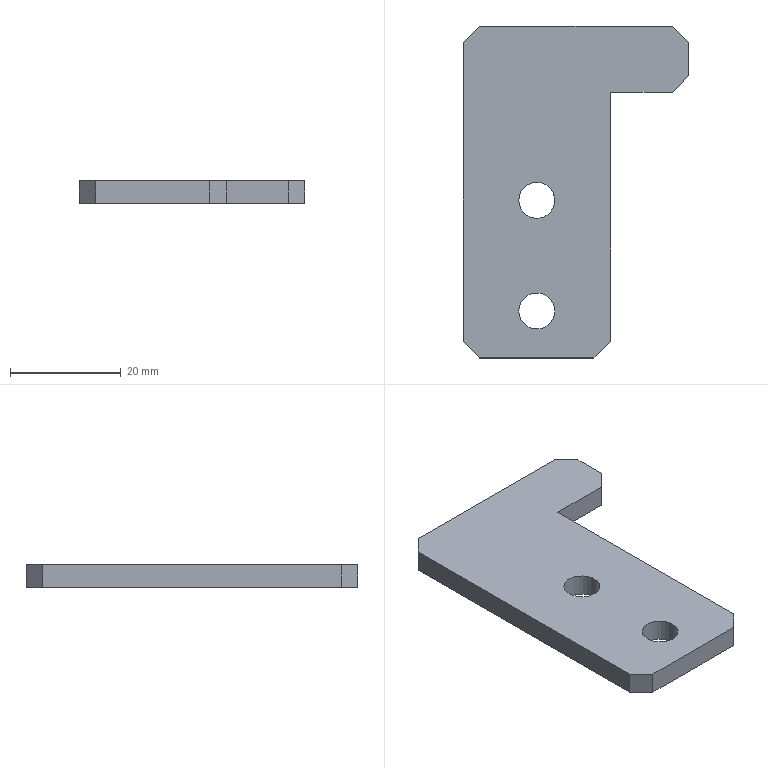Part | STEP file | 64586793 | 1 solid | 17 faces | box 40.84 x 60 x 4 mm | volume 6725 mm3 | plane 13 | cylinder 4 | commonest cylinder face diameters 6.5 x4
STEP:
#1=CARTESIAN_POINT('',(0.,0.,0.));
#2=DIRECTION('',(0.,0.,1.));
#3=DIRECTION('',(1.,0.,0.));
#4=AXIS2_PLACEMENT_3D('',#1,#2,#3);
#5=CARTESIAN_POINT('',(-10.335,0.,0.));
#6=VERTEX_POINT('',#5);
#7=CARTESIAN_POINT('',(10.335,0.,0.));
#8=VERTEX_POINT('',#7);
#9=CARTESIAN_POINT('',(-10.335,0.,0.));
#10=DIRECTION('',(1.,0.,0.));
#11=VECTOR('',#10,1.);
#12=LINE('',#9,#11);
#13=CARTESIAN_POINT('',(0.,0.,0.));
#14=DIRECTION('',(0.,0.,1.));
#15=DIRECTION('',(1.,0.,0.));
#16=AXIS2_PLACEMENT_3D('',#13,#14,#15);
#17=PLANE('',#16);
#18=CARTESIAN_POINT('',(-10.335,0.));
#19=DIRECTION('',(1.,0.));
#20=VECTOR('',#19,1.);
#21=LINE('',#18,#20);
#22=(GEOMETRIC_REPRESENTATION_CONTEXT(2)PARAMETRIC_REPRESENTATION_CONTEXT()REPRESENTATION_CONTEXT('',''));
#23=DEFINITIONAL_REPRESENTATION('',(#21),#22);
#24=PCURVE('',#17,#23);
#25=CARTESIAN_POINT('',(0.,0.,-2.));
#26=DIRECTION('',(0.,-1.,0.));
#27=DIRECTION('',(1.,0.,0.));
#28=AXIS2_PLACEMENT_3D('',#25,#26,#27);
#29=PLANE('',#28);
#30=CARTESIAN_POINT('',(-10.335,2.));
#31=DIRECTION('',(1.,0.));
#32=VECTOR('',#31,1.);
#33=LINE('',#30,#32);
#34=(GEOMETRIC_REPRESENTATION_CONTEXT(2)PARAMETRIC_REPRESENTATION_CONTEXT()REPRESENTATION_CONTEXT('',''));
#35=DEFINITIONAL_REPRESENTATION('',(#33),#34);
#36=PCURVE('',#29,#35);
#37=SURFACE_CURVE('',#12,(#24,#36),.PCURVE_S1.);
#38=EDGE_CURVE('',#6,#8,#37,.T.);
#39=ORIENTED_EDGE('',*,*,#38,.F.);
#40=CARTESIAN_POINT('',(-13.335,3.,0.));
#41=VERTEX_POINT('',#40);
#42=CARTESIAN_POINT('',(-13.335,3.,0.));
#43=DIRECTION('',(0.7071,-0.7071,0.));
#44=VECTOR('',#43,1.);
#45=LINE('',#42,#44);
#46=CARTESIAN_POINT('',(-13.335,3.));
#47=DIRECTION('',(0.7071,-0.7071));
#48=VECTOR('',#47,1.);
#49=LINE('',#46,#48);
#50=(GEOMETRIC_REPRESENTATION_CONTEXT(2)PARAMETRIC_REPRESENTATION_CONTEXT()REPRESENTATION_CONTEXT('',''));
#51=DEFINITIONAL_REPRESENTATION('',(#49),#50);
#52=PCURVE('',#17,#51);
#53=CARTESIAN_POINT('',(-13.335,3.,0.));
#54=DIRECTION('',(-0.7071,-0.7071,0.));
#55=DIRECTION('',(0.,0.,-1.));
#56=AXIS2_PLACEMENT_3D('',#53,#54,#55);
#57=PLANE('',#56);
#58=CARTESIAN_POINT('',(0.,0.));
#59=DIRECTION('',(0.,1.));
#60=VECTOR('',#59,1.);
#61=LINE('',#58,#60);
#62=(GEOMETRIC_REPRESENTATION_CONTEXT(2)PARAMETRIC_REPRESENTATION_CONTEXT()REPRESENTATION_CONTEXT('',''));
#63=DEFINITIONAL_REPRESENTATION('',(#61),#62);
#64=PCURVE('',#57,#63);
#65=SURFACE_CURVE('',#45,(#52,#64),.PCURVE_S1.);
#66=EDGE_CURVE('',#41,#6,#65,.T.);
#67=ORIENTED_EDGE('',*,*,#66,.F.);
#68=CARTESIAN_POINT('',(-13.335,57.,0.));
#69=VERTEX_POINT('',#68);
#70=CARTESIAN_POINT('',(-13.335,57.,0.));
#71=DIRECTION('',(0.,-1.,0.));
#72=VECTOR('',#71,1.);
#73=LINE('',#70,#72);
#74=CARTESIAN_POINT('',(-13.335,57.));
#75=DIRECTION('',(0.,-1.));
#76=VECTOR('',#75,1.);
#77=LINE('',#74,#76);
#78=(GEOMETRIC_REPRESENTATION_CONTEXT(2)PARAMETRIC_REPRESENTATION_CONTEXT()REPRESENTATION_CONTEXT('',''));
#79=DEFINITIONAL_REPRESENTATION('',(#77),#78);
#80=PCURVE('',#17,#79);
#81=CARTESIAN_POINT('',(-13.335,30.,-2.));
#82=DIRECTION('',(-1.,0.,0.));
#83=DIRECTION('',(0.,-1.,0.));
#84=AXIS2_PLACEMENT_3D('',#81,#82,#83);
#85=PLANE('',#84);
#86=CARTESIAN_POINT('',(-27.,2.));
#87=DIRECTION('',(1.,0.));
#88=VECTOR('',#87,1.);
#89=LINE('',#86,#88);
#90=(GEOMETRIC_REPRESENTATION_CONTEXT(2)PARAMETRIC_REPRESENTATION_CONTEXT()REPRESENTATION_CONTEXT('',''));
#91=DEFINITIONAL_REPRESENTATION('',(#89),#90);
#92=PCURVE('',#85,#91);
#93=SURFACE_CURVE('',#73,(#80,#92),.PCURVE_S1.);
#94=EDGE_CURVE('',#69,#41,#93,.T.);
#95=ORIENTED_EDGE('',*,*,#94,.F.);
#96=CARTESIAN_POINT('',(-10.335,60.,0.));
#97=VERTEX_POINT('',#96);
#98=CARTESIAN_POINT('',(-10.335,60.,0.));
#99=DIRECTION('',(-0.7071,-0.7071,0.));
#100=VECTOR('',#99,1.);
#101=LINE('',#98,#100);
#102=CARTESIAN_POINT('',(-10.335,60.));
#103=DIRECTION('',(-0.7071,-0.7071));
#104=VECTOR('',#103,1.);
#105=LINE('',#102,#104);
#106=(GEOMETRIC_REPRESENTATION_CONTEXT(2)PARAMETRIC_REPRESENTATION_CONTEXT()REPRESENTATION_CONTEXT('',''));
#107=DEFINITIONAL_REPRESENTATION('',(#105),#106);
#108=PCURVE('',#17,#107);
#109=CARTESIAN_POINT('',(-10.335,60.,0.));
#110=DIRECTION('',(-0.7071,0.7071,0.));
#111=DIRECTION('',(0.,0.,-1.));
#112=AXIS2_PLACEMENT_3D('',#109,#110,#111);
#113=PLANE('',#112);
#114=CARTESIAN_POINT('',(0.,0.));
#115=DIRECTION('',(0.,1.));
#116=VECTOR('',#115,1.);
#117=LINE('',#114,#116);
#118=(GEOMETRIC_REPRESENTATION_CONTEXT(2)PARAMETRIC_REPRESENTATION_CONTEXT()REPRESENTATION_CONTEXT('',''));
#119=DEFINITIONAL_REPRESENTATION('',(#117),#118);
#120=PCURVE('',#113,#119);
#121=SURFACE_CURVE('',#101,(#108,#120),.PCURVE_S1.);
#122=EDGE_CURVE('',#97,#69,#121,.T.);
#123=ORIENTED_EDGE('',*,*,#122,.F.);
#124=CARTESIAN_POINT('',(24.505,60.,0.));
#125=VERTEX_POINT('',#124);
#126=CARTESIAN_POINT('',(24.505,60.,0.));
#127=DIRECTION('',(-1.,0.,0.));
#128=VECTOR('',#127,1.);
#129=LINE('',#126,#128);
#130=CARTESIAN_POINT('',(24.505,60.));
#131=DIRECTION('',(-1.,0.));
#132=VECTOR('',#131,1.);
#133=LINE('',#130,#132);
#134=(GEOMETRIC_REPRESENTATION_CONTEXT(2)PARAMETRIC_REPRESENTATION_CONTEXT()REPRESENTATION_CONTEXT('',''));
#135=DEFINITIONAL_REPRESENTATION('',(#133),#134);
#136=PCURVE('',#17,#135);
#137=CARTESIAN_POINT('',(7.085,60.,-2.));
#138=DIRECTION('',(0.,1.,0.));
#139=DIRECTION('',(-1.,0.,0.));
#140=AXIS2_PLACEMENT_3D('',#137,#138,#139);
#141=PLANE('',#140);
#142=CARTESIAN_POINT('',(-17.42,2.));
#143=DIRECTION('',(1.,0.));
#144=VECTOR('',#143,1.);
#145=LINE('',#142,#144);
#146=(GEOMETRIC_REPRESENTATION_CONTEXT(2)PARAMETRIC_REPRESENTATION_CONTEXT()REPRESENTATION_CONTEXT('',''));
#147=DEFINITIONAL_REPRESENTATION('',(#145),#146);
#148=PCURVE('',#141,#147);
#149=SURFACE_CURVE('',#129,(#136,#148),.PCURVE_S1.);
#150=EDGE_CURVE('',#125,#97,#149,.T.);
#151=ORIENTED_EDGE('',*,*,#150,.F.);
#152=CARTESIAN_POINT('',(27.505,57.,0.));
#153=VERTEX_POINT('',#152);
#154=CARTESIAN_POINT('',(27.505,57.,0.));
#155=DIRECTION('',(-0.7071,0.7071,0.));
#156=VECTOR('',#155,1.);
#157=LINE('',#154,#156);
#158=CARTESIAN_POINT('',(27.505,57.));
#159=DIRECTION('',(-0.7071,0.7071));
#160=VECTOR('',#159,1.);
#161=LINE('',#158,#160);
#162=(GEOMETRIC_REPRESENTATION_CONTEXT(2)PARAMETRIC_REPRESENTATION_CONTEXT()REPRESENTATION_CONTEXT('',''));
#163=DEFINITIONAL_REPRESENTATION('',(#161),#162);
#164=PCURVE('',#17,#163);
#165=CARTESIAN_POINT('',(27.505,57.,0.));
#166=DIRECTION('',(0.7071,0.7071,0.));
#167=DIRECTION('',(0.,0.,-1.));
#168=AXIS2_PLACEMENT_3D('',#165,#166,#167);
#169=PLANE('',#168);
#170=CARTESIAN_POINT('',(0.,0.));
#171=DIRECTION('',(0.,1.));
#172=VECTOR('',#171,1.);
#173=LINE('',#170,#172);
#174=(GEOMETRIC_REPRESENTATION_CONTEXT(2)PARAMETRIC_REPRESENTATION_CONTEXT()REPRESENTATION_CONTEXT('',''));
#175=DEFINITIONAL_REPRESENTATION('',(#173),#174);
#176=PCURVE('',#169,#175);
#177=SURFACE_CURVE('',#157,(#164,#176),.PCURVE_S1.);
#178=EDGE_CURVE('',#153,#125,#177,.T.);
#179=ORIENTED_EDGE('',*,*,#178,.F.);
#180=CARTESIAN_POINT('',(27.505,51.,0.));
#181=VERTEX_POINT('',#180);
#182=CARTESIAN_POINT('',(27.505,51.,0.));
#183=DIRECTION('',(0.,1.,0.));
#184=VECTOR('',#183,1.);
#185=LINE('',#182,#184);
#186=CARTESIAN_POINT('',(27.505,51.));
#187=DIRECTION('',(0.,1.));
#188=VECTOR('',#187,1.);
#189=LINE('',#186,#188);
#190=(GEOMETRIC_REPRESENTATION_CONTEXT(2)PARAMETRIC_REPRESENTATION_CONTEXT()REPRESENTATION_CONTEXT('',''));
#191=DEFINITIONAL_REPRESENTATION('',(#189),#190);
#192=PCURVE('',#17,#191);
#193=CARTESIAN_POINT('',(27.505,54.,-2.));
#194=DIRECTION('',(1.,0.,0.));
#195=DIRECTION('',(0.,1.,0.));
#196=AXIS2_PLACEMENT_3D('',#193,#194,#195);
#197=PLANE('',#196);
#198=CARTESIAN_POINT('',(-3.,2.));
#199=DIRECTION('',(1.,0.));
#200=VECTOR('',#199,1.);
#201=LINE('',#198,#200);
#202=(GEOMETRIC_REPRESENTATION_CONTEXT(2)PARAMETRIC_REPRESENTATION_CONTEXT()REPRESENTATION_CONTEXT('',''));
#203=DEFINITIONAL_REPRESENTATION('',(#201),#202);
#204=PCURVE('',#197,#203);
#205=SURFACE_CURVE('',#185,(#192,#204),.PCURVE_S1.);
#206=EDGE_CURVE('',#181,#153,#205,.T.);
#207=ORIENTED_EDGE('',*,*,#206,.F.);
#208=CARTESIAN_POINT('',(24.505,48.,0.));
#209=VERTEX_POINT('',#208);
#210=CARTESIAN_POINT('',(24.505,48.,0.));
#211=DIRECTION('',(0.7071,0.7071,0.));
#212=VECTOR('',#211,1.);
#213=LINE('',#210,#212);
#214=CARTESIAN_POINT('',(24.505,48.));
#215=DIRECTION('',(0.7071,0.7071));
#216=VECTOR('',#215,1.);
#217=LINE('',#214,#216);
#218=(GEOMETRIC_REPRESENTATION_CONTEXT(2)PARAMETRIC_REPRESENTATION_CONTEXT()REPRESENTATION_CONTEXT('',''));
#219=DEFINITIONAL_REPRESENTATION('',(#217),#218);
#220=PCURVE('',#17,#219);
#221=CARTESIAN_POINT('',(24.505,48.,0.));
#222=DIRECTION('',(0.7071,-0.7071,0.));
#223=DIRECTION('',(0.,0.,-1.));
#224=AXIS2_PLACEMENT_3D('',#221,#222,#223);
#225=PLANE('',#224);
#226=CARTESIAN_POINT('',(0.,0.));
#227=DIRECTION('',(0.,1.));
#228=VECTOR('',#227,1.);
#229=LINE('',#226,#228);
#230=(GEOMETRIC_REPRESENTATION_CONTEXT(2)PARAMETRIC_REPRESENTATION_CONTEXT()REPRESENTATION_CONTEXT('',''));
#231=DEFINITIONAL_REPRESENTATION('',(#229),#230);
#232=PCURVE('',#225,#231);
#233=SURFACE_CURVE('',#213,(#220,#232),.PCURVE_S1.);
#234=EDGE_CURVE('',#209,#181,#233,.T.);
#235=ORIENTED_EDGE('',*,*,#234,.F.);
#236=CARTESIAN_POINT('',(13.335,48.,0.));
#237=VERTEX_POINT('',#236);
#238=CARTESIAN_POINT('',(13.335,48.,0.));
#239=DIRECTION('',(1.,0.,0.));
#240=VECTOR('',#239,1.);
#241=LINE('',#238,#240);
#242=CARTESIAN_POINT('',(13.335,48.));
#243=DIRECTION('',(1.,0.));
#244=VECTOR('',#243,1.);
#245=LINE('',#242,#244);
#246=(GEOMETRIC_REPRESENTATION_CONTEXT(2)PARAMETRIC_REPRESENTATION_CONTEXT()REPRESENTATION_CONTEXT('',''));
#247=DEFINITIONAL_REPRESENTATION('',(#245),#246);
#248=PCURVE('',#17,#247);
#249=CARTESIAN_POINT('',(20.42,48.,-2.));
#250=DIRECTION('',(0.,-1.,0.));
#251=DIRECTION('',(1.,0.,0.));
#252=AXIS2_PLACEMENT_3D('',#249,#250,#251);
#253=PLANE('',#252);
#254=CARTESIAN_POINT('',(-7.085,2.));
#255=DIRECTION('',(1.,0.));
#256=VECTOR('',#255,1.);
#257=LINE('',#254,#256);
#258=(GEOMETRIC_REPRESENTATION_CONTEXT(2)PARAMETRIC_REPRESENTATION_CONTEXT()REPRESENTATION_CONTEXT('',''));
#259=DEFINITIONAL_REPRESENTATION('',(#257),#258);
#260=PCURVE('',#253,#259);
#261=SURFACE_CURVE('',#241,(#248,#260),.PCURVE_S1.);
#262=EDGE_CURVE('',#237,#209,#261,.T.);
#263=ORIENTED_EDGE('',*,*,#262,.F.);
#264=CARTESIAN_POINT('',(13.335,3.,0.));
#265=VERTEX_POINT('',#264);
#266=CARTESIAN_POINT('',(13.335,3.,0.));
#267=DIRECTION('',(0.,1.,0.));
#268=VECTOR('',#267,1.);
#269=LINE('',#266,#268);
#270=CARTESIAN_POINT('',(13.335,3.));
#271=DIRECTION('',(0.,1.));
#272=VECTOR('',#271,1.);
#273=LINE('',#270,#272);
#274=(GEOMETRIC_REPRESENTATION_CONTEXT(2)PARAMETRIC_REPRESENTATION_CONTEXT()REPRESENTATION_CONTEXT('',''));
#275=DEFINITIONAL_REPRESENTATION('',(#273),#274);
#276=PCURVE('',#17,#275);
#277=CARTESIAN_POINT('',(13.335,24.,-2.));
#278=DIRECTION('',(1.,0.,0.));
#279=DIRECTION('',(0.,1.,0.));
#280=AXIS2_PLACEMENT_3D('',#277,#278,#279);
#281=PLANE('',#280);
#282=CARTESIAN_POINT('',(-21.,2.));
#283=DIRECTION('',(1.,0.));
#284=VECTOR('',#283,1.);
#285=LINE('',#282,#284);
#286=(GEOMETRIC_REPRESENTATION_CONTEXT(2)PARAMETRIC_REPRESENTATION_CONTEXT()REPRESENTATION_CONTEXT('',''));
#287=DEFINITIONAL_REPRESENTATION('',(#285),#286);
#288=PCURVE('',#281,#287);
#289=SURFACE_CURVE('',#269,(#276,#288),.PCURVE_S1.);
#290=EDGE_CURVE('',#265,#237,#289,.T.);
#291=ORIENTED_EDGE('',*,*,#290,.F.);
#292=CARTESIAN_POINT('',(10.335,0.,0.));
#293=DIRECTION('',(0.7071,0.7071,0.));
#294=VECTOR('',#293,1.);
#295=LINE('',#292,#294);
#296=CARTESIAN_POINT('',(10.335,0.));
#297=DIRECTION('',(0.7071,0.7071));
#298=VECTOR('',#297,1.);
#299=LINE('',#296,#298);
#300=(GEOMETRIC_REPRESENTATION_CONTEXT(2)PARAMETRIC_REPRESENTATION_CONTEXT()REPRESENTATION_CONTEXT('',''));
#301=DEFINITIONAL_REPRESENTATION('',(#299),#300);
#302=PCURVE('',#17,#301);
#303=CARTESIAN_POINT('',(10.335,0.,0.));
#304=DIRECTION('',(0.7071,-0.7071,0.));
#305=DIRECTION('',(0.,0.,-1.));
#306=AXIS2_PLACEMENT_3D('',#303,#304,#305);
#307=PLANE('',#306);
#308=CARTESIAN_POINT('',(0.,0.));
#309=DIRECTION('',(0.,1.));
#310=VECTOR('',#309,1.);
#311=LINE('',#308,#310);
#312=(GEOMETRIC_REPRESENTATION_CONTEXT(2)PARAMETRIC_REPRESENTATION_CONTEXT()REPRESENTATION_CONTEXT('',''));
#313=DEFINITIONAL_REPRESENTATION('',(#311),#312);
#314=PCURVE('',#307,#313);
#315=SURFACE_CURVE('',#295,(#302,#314),.PCURVE_S1.);
#316=EDGE_CURVE('',#8,#265,#315,.T.);
#317=ORIENTED_EDGE('',*,*,#316,.F.);
#318=EDGE_LOOP('',(#39,#67,#95,#123,#151,#179,#207,#235,#263,#291,#317));
#319=FACE_BOUND('',#318,.F.);
#320=CARTESIAN_POINT('',(-3.25,28.5,0.));
#321=VERTEX_POINT('',#320);
#322=CARTESIAN_POINT('',(3.25,28.5,0.));
#323=VERTEX_POINT('',#322);
#324=CARTESIAN_POINT('',(0.,28.5,0.));
#325=DIRECTION('',(0.,0.,1.));
#326=DIRECTION('',(-1.,0.,0.));
#327=AXIS2_PLACEMENT_3D('',#324,#325,#326);
#328=CIRCLE('',#327,3.25);
#329=CARTESIAN_POINT('',(0.,28.5));
#330=DIRECTION('',(-1.,0.));
#331=AXIS2_PLACEMENT_2D('',#329,#330);
#332=CIRCLE('',#331,3.25);
#333=(GEOMETRIC_REPRESENTATION_CONTEXT(2)PARAMETRIC_REPRESENTATION_CONTEXT()REPRESENTATION_CONTEXT('',''));
#334=DEFINITIONAL_REPRESENTATION('',(#332),#333);
#335=PCURVE('',#17,#334);
#336=CARTESIAN_POINT('',(0.,28.5,-2.));
#337=DIRECTION('',(0.,0.,1.));
#338=DIRECTION('',(-1.,0.,0.));
#339=AXIS2_PLACEMENT_3D('',#336,#337,#338);
#340=CYLINDRICAL_SURFACE('',#339,3.25);
#341=CARTESIAN_POINT('',(0.,2.));
#342=DIRECTION('',(1.,0.));
#343=VECTOR('',#342,1.);
#344=LINE('',#341,#343);
#345=(GEOMETRIC_REPRESENTATION_CONTEXT(2)PARAMETRIC_REPRESENTATION_CONTEXT()REPRESENTATION_CONTEXT('',''));
#346=DEFINITIONAL_REPRESENTATION('',(#344),#345);
#347=PCURVE('',#340,#346);
#348=SURFACE_CURVE('',#328,(#335,#347),.PCURVE_S1.);
#349=EDGE_CURVE('',#321,#323,#348,.T.);
#350=ORIENTED_EDGE('',*,*,#349,.T.);
#351=CARTESIAN_POINT('',(0.,28.5,0.));
#352=DIRECTION('',(0.,0.,1.));
#353=DIRECTION('',(1.,0.,0.));
#354=AXIS2_PLACEMENT_3D('',#351,#352,#353);
#355=CIRCLE('',#354,3.25);
#356=CARTESIAN_POINT('',(0.,28.5));
#357=DIRECTION('',(1.,0.));
#358=AXIS2_PLACEMENT_2D('',#356,#357);
#359=CIRCLE('',#358,3.25);
#360=(GEOMETRIC_REPRESENTATION_CONTEXT(2)PARAMETRIC_REPRESENTATION_CONTEXT()REPRESENTATION_CONTEXT('',''));
#361=DEFINITIONAL_REPRESENTATION('',(#359),#360);
#362=PCURVE('',#17,#361);
#363=CARTESIAN_POINT('',(0.,28.5,-2.));
#364=DIRECTION('',(0.,0.,1.));
#365=DIRECTION('',(1.,0.,0.));
#366=AXIS2_PLACEMENT_3D('',#363,#364,#365);
#367=CYLINDRICAL_SURFACE('',#366,3.25);
#368=CARTESIAN_POINT('',(0.,2.));
#369=DIRECTION('',(1.,0.));
#370=VECTOR('',#369,1.);
#371=LINE('',#368,#370);
#372=(GEOMETRIC_REPRESENTATION_CONTEXT(2)PARAMETRIC_REPRESENTATION_CONTEXT()REPRESENTATION_CONTEXT('',''));
#373=DEFINITIONAL_REPRESENTATION('',(#371),#372);
#374=PCURVE('',#367,#373);
#375=SURFACE_CURVE('',#355,(#362,#374),.PCURVE_S1.);
#376=EDGE_CURVE('',#323,#321,#375,.T.);
#377=ORIENTED_EDGE('',*,*,#376,.T.);
#378=EDGE_LOOP('',(#350,#377));
#379=FACE_BOUND('',#378,.F.);
#380=CARTESIAN_POINT('',(-3.25,8.5,0.));
#381=VERTEX_POINT('',#380);
#382=CARTESIAN_POINT('',(3.25,8.5,0.));
#383=VERTEX_POINT('',#382);
#384=CARTESIAN_POINT('',(0.,8.5,0.));
#385=DIRECTION('',(0.,0.,1.));
#386=DIRECTION('',(-1.,0.,0.));
#387=AXIS2_PLACEMENT_3D('',#384,#385,#386);
#388=CIRCLE('',#387,3.25);
#389=CARTESIAN_POINT('',(0.,8.5));
#390=DIRECTION('',(-1.,0.));
#391=AXIS2_PLACEMENT_2D('',#389,#390);
#392=CIRCLE('',#391,3.25);
#393=(GEOMETRIC_REPRESENTATION_CONTEXT(2)PARAMETRIC_REPRESENTATION_CONTEXT()REPRESENTATION_CONTEXT('',''));
#394=DEFINITIONAL_REPRESENTATION('',(#392),#393);
#395=PCURVE('',#17,#394);
#396=CARTESIAN_POINT('',(0.,8.5,-2.));
#397=DIRECTION('',(0.,0.,1.));
#398=DIRECTION('',(-1.,0.,0.));
#399=AXIS2_PLACEMENT_3D('',#396,#397,#398);
#400=CYLINDRICAL_SURFACE('',#399,3.25);
#401=CARTESIAN_POINT('',(0.,2.));
#402=DIRECTION('',(1.,0.));
#403=VECTOR('',#402,1.);
#404=LINE('',#401,#403);
#405=(GEOMETRIC_REPRESENTATION_CONTEXT(2)PARAMETRIC_REPRESENTATION_CONTEXT()REPRESENTATION_CONTEXT('',''));
#406=DEFINITIONAL_REPRESENTATION('',(#404),#405);
#407=PCURVE('',#400,#406);
#408=SURFACE_CURVE('',#388,(#395,#407),.PCURVE_S1.);
#409=EDGE_CURVE('',#381,#383,#408,.T.);
#410=ORIENTED_EDGE('',*,*,#409,.T.);
#411=CARTESIAN_POINT('',(0.,8.5,0.));
#412=DIRECTION('',(0.,0.,1.));
#413=DIRECTION('',(1.,0.,0.));
#414=AXIS2_PLACEMENT_3D('',#411,#412,#413);
#415=CIRCLE('',#414,3.25);
#416=CARTESIAN_POINT('',(0.,8.5));
#417=DIRECTION('',(1.,0.));
#418=AXIS2_PLACEMENT_2D('',#416,#417);
#419=CIRCLE('',#418,3.25);
#420=(GEOMETRIC_REPRESENTATION_CONTEXT(2)PARAMETRIC_REPRESENTATION_CONTEXT()REPRESENTATION_CONTEXT('',''));
#421=DEFINITIONAL_REPRESENTATION('',(#419),#420);
#422=PCURVE('',#17,#421);
#423=CARTESIAN_POINT('',(0.,8.5,-2.));
#424=DIRECTION('',(0.,0.,1.));
#425=DIRECTION('',(1.,0.,0.));
#426=AXIS2_PLACEMENT_3D('',#423,#424,#425);
#427=CYLINDRICAL_SURFACE('',#426,3.25);
#428=CARTESIAN_POINT('',(0.,2.));
#429=DIRECTION('',(1.,0.));
#430=VECTOR('',#429,1.);
#431=LINE('',#428,#430);
#432=(GEOMETRIC_REPRESENTATION_CONTEXT(2)PARAMETRIC_REPRESENTATION_CONTEXT()REPRESENTATION_CONTEXT('',''));
#433=DEFINITIONAL_REPRESENTATION('',(#431),#432);
#434=PCURVE('',#427,#433);
#435=SURFACE_CURVE('',#415,(#422,#434),.PCURVE_S1.);
#436=EDGE_CURVE('',#383,#381,#435,.T.);
#437=ORIENTED_EDGE('',*,*,#436,.T.);
#438=EDGE_LOOP('',(#410,#437));
#439=FACE_BOUND('',#438,.F.);
#440=ADVANCED_FACE('',(#319,#379,#439),#17,.T.);
#441=ORIENTED_EDGE('',*,*,#38,.T.);
#442=CARTESIAN_POINT('',(10.335,0.,-4.));
#443=VERTEX_POINT('',#442);
#444=CARTESIAN_POINT('',(10.335,0.,0.));
#445=DIRECTION('',(0.,0.,-1.));
#446=VECTOR('',#445,1.);
#447=LINE('',#444,#446);
#448=CARTESIAN_POINT('',(10.335,2.));
#449=DIRECTION('',(0.,-1.));
#450=VECTOR('',#449,1.);
#451=LINE('',#448,#450);
#452=(GEOMETRIC_REPRESENTATION_CONTEXT(2)PARAMETRIC_REPRESENTATION_CONTEXT()REPRESENTATION_CONTEXT('',''));
#453=DEFINITIONAL_REPRESENTATION('',(#451),#452);
#454=PCURVE('',#29,#453);
#455=CARTESIAN_POINT('',(0.,0.));
#456=DIRECTION('',(1.,0.));
#457=VECTOR('',#456,1.);
#458=LINE('',#455,#457);
#459=(GEOMETRIC_REPRESENTATION_CONTEXT(2)PARAMETRIC_REPRESENTATION_CONTEXT()REPRESENTATION_CONTEXT('',''));
#460=DEFINITIONAL_REPRESENTATION('',(#458),#459);
#461=PCURVE('',#307,#460);
#462=SURFACE_CURVE('',#447,(#454,#461),.PCURVE_S1.);
#463=EDGE_CURVE('',#8,#443,#462,.T.);
#464=ORIENTED_EDGE('',*,*,#463,.T.);
#465=CARTESIAN_POINT('',(-10.335,0.,-4.));
#466=VERTEX_POINT('',#465);
#467=CARTESIAN_POINT('',(-10.335,0.,-4.));
#468=DIRECTION('',(1.,0.,0.));
#469=VECTOR('',#468,1.);
#470=LINE('',#467,#469);
#471=CARTESIAN_POINT('',(-10.335,-2.));
#472=DIRECTION('',(1.,0.));
#473=VECTOR('',#472,1.);
#474=LINE('',#471,#473);
#475=(GEOMETRIC_REPRESENTATION_CONTEXT(2)PARAMETRIC_REPRESENTATION_CONTEXT()REPRESENTATION_CONTEXT('',''));
#476=DEFINITIONAL_REPRESENTATION('',(#474),#475);
#477=PCURVE('',#29,#476);
#478=CARTESIAN_POINT('',(0.,0.,-4.));
#479=DIRECTION('',(0.,0.,1.));
#480=DIRECTION('',(1.,0.,0.));
#481=AXIS2_PLACEMENT_3D('',#478,#479,#480);
#482=PLANE('',#481);
#483=CARTESIAN_POINT('',(-10.335,0.));
#484=DIRECTION('',(1.,0.));
#485=VECTOR('',#484,1.);
#486=LINE('',#483,#485);
#487=(GEOMETRIC_REPRESENTATION_CONTEXT(2)PARAMETRIC_REPRESENTATION_CONTEXT()REPRESENTATION_CONTEXT('',''));
#488=DEFINITIONAL_REPRESENTATION('',(#486),#487);
#489=PCURVE('',#482,#488);
#490=SURFACE_CURVE('',#470,(#477,#489),.PCURVE_S1.);
#491=EDGE_CURVE('',#466,#443,#490,.T.);
#492=ORIENTED_EDGE('',*,*,#491,.F.);
#493=CARTESIAN_POINT('',(-10.335,0.,0.));
#494=DIRECTION('',(0.,0.,-1.));
#495=VECTOR('',#494,1.);
#496=LINE('',#493,#495);
#497=CARTESIAN_POINT('',(-10.335,2.));
#498=DIRECTION('',(0.,-1.));
#499=VECTOR('',#498,1.);
#500=LINE('',#497,#499);
#501=(GEOMETRIC_REPRESENTATION_CONTEXT(2)PARAMETRIC_REPRESENTATION_CONTEXT()REPRESENTATION_CONTEXT('',''));
#502=DEFINITIONAL_REPRESENTATION('',(#500),#501);
#503=PCURVE('',#29,#502);
#504=CARTESIAN_POINT('',(0.,4.243));
#505=DIRECTION('',(1.,0.));
#506=VECTOR('',#505,1.);
#507=LINE('',#504,#506);
#508=(GEOMETRIC_REPRESENTATION_CONTEXT(2)PARAMETRIC_REPRESENTATION_CONTEXT()REPRESENTATION_CONTEXT('',''));
#509=DEFINITIONAL_REPRESENTATION('',(#507),#508);
#510=PCURVE('',#57,#509);
#511=SURFACE_CURVE('',#496,(#503,#510),.PCURVE_S1.);
#512=EDGE_CURVE('',#6,#466,#511,.T.);
#513=ORIENTED_EDGE('',*,*,#512,.F.);
#514=EDGE_LOOP('',(#441,#464,#492,#513));
#515=FACE_BOUND('',#514,.F.);
#516=ADVANCED_FACE('',(#515),#29,.T.);
#517=ORIENTED_EDGE('',*,*,#463,.F.);
#518=ORIENTED_EDGE('',*,*,#316,.T.);
#519=CARTESIAN_POINT('',(13.335,3.,-4.));
#520=VERTEX_POINT('',#519);
#521=CARTESIAN_POINT('',(13.335,3.,0.));
#522=DIRECTION('',(0.,0.,-1.));
#523=VECTOR('',#522,1.);
#524=LINE('',#521,#523);
#525=CARTESIAN_POINT('',(0.,4.243));
#526=DIRECTION('',(1.,0.));
#527=VECTOR('',#526,1.);
#528=LINE('',#525,#527);
#529=(GEOMETRIC_REPRESENTATION_CONTEXT(2)PARAMETRIC_REPRESENTATION_CONTEXT()REPRESENTATION_CONTEXT('',''));
#530=DEFINITIONAL_REPRESENTATION('',(#528),#529);
#531=PCURVE('',#307,#530);
#532=CARTESIAN_POINT('',(-21.,2.));
#533=DIRECTION('',(0.,-1.));
#534=VECTOR('',#533,1.);
#535=LINE('',#532,#534);
#536=(GEOMETRIC_REPRESENTATION_CONTEXT(2)PARAMETRIC_REPRESENTATION_CONTEXT()REPRESENTATION_CONTEXT('',''));
#537=DEFINITIONAL_REPRESENTATION('',(#535),#536);
#538=PCURVE('',#281,#537);
#539=SURFACE_CURVE('',#524,(#531,#538),.PCURVE_S1.);
#540=EDGE_CURVE('',#265,#520,#539,.T.);
#541=ORIENTED_EDGE('',*,*,#540,.T.);
#542=CARTESIAN_POINT('',(10.335,0.,-4.));
#543=DIRECTION('',(0.7071,0.7071,0.));
#544=VECTOR('',#543,1.);
#545=LINE('',#542,#544);
#546=CARTESIAN_POINT('',(4.,0.));
#547=DIRECTION('',(0.,1.));
#548=VECTOR('',#547,1.);
#549=LINE('',#546,#548);
#550=(GEOMETRIC_REPRESENTATION_CONTEXT(2)PARAMETRIC_REPRESENTATION_CONTEXT()REPRESENTATION_CONTEXT('',''));
#551=DEFINITIONAL_REPRESENTATION('',(#549),#550);
#552=PCURVE('',#307,#551);
#553=CARTESIAN_POINT('',(10.335,0.));
#554=DIRECTION('',(0.7071,0.7071));
#555=VECTOR('',#554,1.);
#556=LINE('',#553,#555);
#557=(GEOMETRIC_REPRESENTATION_CONTEXT(2)PARAMETRIC_REPRESENTATION_CONTEXT()REPRESENTATION_CONTEXT('',''));
#558=DEFINITIONAL_REPRESENTATION('',(#556),#557);
#559=PCURVE('',#482,#558);
#560=SURFACE_CURVE('',#545,(#552,#559),.PCURVE_S1.);
#561=EDGE_CURVE('',#443,#520,#560,.T.);
#562=ORIENTED_EDGE('',*,*,#561,.F.);
#563=EDGE_LOOP('',(#517,#518,#541,#562));
#564=FACE_BOUND('',#563,.F.);
#565=ADVANCED_FACE('',(#564),#307,.T.);
#566=ORIENTED_EDGE('',*,*,#290,.T.);
#567=CARTESIAN_POINT('',(13.335,48.,-4.));
#568=VERTEX_POINT('',#567);
#569=CARTESIAN_POINT('',(13.335,48.,0.));
#570=DIRECTION('',(0.,0.,-1.));
#571=VECTOR('',#570,1.);
#572=LINE('',#569,#571);
#573=CARTESIAN_POINT('',(24.,2.));
#574=DIRECTION('',(0.,-1.));
#575=VECTOR('',#574,1.);
#576=LINE('',#573,#575);
#577=(GEOMETRIC_REPRESENTATION_CONTEXT(2)PARAMETRIC_REPRESENTATION_CONTEXT()REPRESENTATION_CONTEXT('',''));
#578=DEFINITIONAL_REPRESENTATION('',(#576),#577);
#579=PCURVE('',#281,#578);
#580=CARTESIAN_POINT('',(-7.085,2.));
#581=DIRECTION('',(0.,-1.));
#582=VECTOR('',#581,1.);
#583=LINE('',#580,#582);
#584=(GEOMETRIC_REPRESENTATION_CONTEXT(2)PARAMETRIC_REPRESENTATION_CONTEXT()REPRESENTATION_CONTEXT('',''));
#585=DEFINITIONAL_REPRESENTATION('',(#583),#584);
#586=PCURVE('',#253,#585);
#587=SURFACE_CURVE('',#572,(#579,#586),.PCURVE_S1.);
#588=EDGE_CURVE('',#237,#568,#587,.T.);
#589=ORIENTED_EDGE('',*,*,#588,.T.);
#590=CARTESIAN_POINT('',(13.335,3.,-4.));
#591=DIRECTION('',(0.,1.,0.));
#592=VECTOR('',#591,1.);
#593=LINE('',#590,#592);
#594=CARTESIAN_POINT('',(-21.,-2.));
#595=DIRECTION('',(1.,0.));
#596=VECTOR('',#595,1.);
#597=LINE('',#594,#596);
#598=(GEOMETRIC_REPRESENTATION_CONTEXT(2)PARAMETRIC_REPRESENTATION_CONTEXT()REPRESENTATION_CONTEXT('',''));
#599=DEFINITIONAL_REPRESENTATION('',(#597),#598);
#600=PCURVE('',#281,#599);
#601=CARTESIAN_POINT('',(13.335,3.));
#602=DIRECTION('',(0.,1.));
#603=VECTOR('',#602,1.);
#604=LINE('',#601,#603);
#605=(GEOMETRIC_REPRESENTATION_CONTEXT(2)PARAMETRIC_REPRESENTATION_CONTEXT()REPRESENTATION_CONTEXT('',''));
#606=DEFINITIONAL_REPRESENTATION('',(#604),#605);
#607=PCURVE('',#482,#606);
#608=SURFACE_CURVE('',#593,(#600,#607),.PCURVE_S1.);
#609=EDGE_CURVE('',#520,#568,#608,.T.);
#610=ORIENTED_EDGE('',*,*,#609,.F.);
#611=ORIENTED_EDGE('',*,*,#540,.F.);
#612=EDGE_LOOP('',(#566,#589,#610,#611));
#613=FACE_BOUND('',#612,.F.);
#614=ADVANCED_FACE('',(#613),#281,.T.);
#615=ORIENTED_EDGE('',*,*,#262,.T.);
#616=CARTESIAN_POINT('',(24.505,48.,-4.));
#617=VERTEX_POINT('',#616);
#618=CARTESIAN_POINT('',(24.505,48.,0.));
#619=DIRECTION('',(0.,0.,-1.));
#620=VECTOR('',#619,1.);
#621=LINE('',#618,#620);
#622=CARTESIAN_POINT('',(4.085,2.));
#623=DIRECTION('',(0.,-1.));
#624=VECTOR('',#623,1.);
#625=LINE('',#622,#624);
#626=(GEOMETRIC_REPRESENTATION_CONTEXT(2)PARAMETRIC_REPRESENTATION_CONTEXT()REPRESENTATION_CONTEXT('',''));
#627=DEFINITIONAL_REPRESENTATION('',(#625),#626);
#628=PCURVE('',#253,#627);
#629=CARTESIAN_POINT('',(0.,0.));
#630=DIRECTION('',(1.,0.));
#631=VECTOR('',#630,1.);
#632=LINE('',#629,#631);
#633=(GEOMETRIC_REPRESENTATION_CONTEXT(2)PARAMETRIC_REPRESENTATION_CONTEXT()REPRESENTATION_CONTEXT('',''));
#634=DEFINITIONAL_REPRESENTATION('',(#632),#633);
#635=PCURVE('',#225,#634);
#636=SURFACE_CURVE('',#621,(#628,#635),.PCURVE_S1.);
#637=EDGE_CURVE('',#209,#617,#636,.T.);
#638=ORIENTED_EDGE('',*,*,#637,.T.);
#639=CARTESIAN_POINT('',(13.335,48.,-4.));
#640=DIRECTION('',(1.,0.,0.));
#641=VECTOR('',#640,1.);
#642=LINE('',#639,#641);
#643=CARTESIAN_POINT('',(-7.085,-2.));
#644=DIRECTION('',(1.,0.));
#645=VECTOR('',#644,1.);
#646=LINE('',#643,#645);
#647=(GEOMETRIC_REPRESENTATION_CONTEXT(2)PARAMETRIC_REPRESENTATION_CONTEXT()REPRESENTATION_CONTEXT('',''));
#648=DEFINITIONAL_REPRESENTATION('',(#646),#647);
#649=PCURVE('',#253,#648);
#650=CARTESIAN_POINT('',(13.335,48.));
#651=DIRECTION('',(1.,0.));
#652=VECTOR('',#651,1.);
#653=LINE('',#650,#652);
#654=(GEOMETRIC_REPRESENTATION_CONTEXT(2)PARAMETRIC_REPRESENTATION_CONTEXT()REPRESENTATION_CONTEXT('',''));
#655=DEFINITIONAL_REPRESENTATION('',(#653),#654);
#656=PCURVE('',#482,#655);
#657=SURFACE_CURVE('',#642,(#649,#656),.PCURVE_S1.);
#658=EDGE_CURVE('',#568,#617,#657,.T.);
#659=ORIENTED_EDGE('',*,*,#658,.F.);
#660=ORIENTED_EDGE('',*,*,#588,.F.);
#661=EDGE_LOOP('',(#615,#638,#659,#660));
#662=FACE_BOUND('',#661,.F.);
#663=ADVANCED_FACE('',(#662),#253,.T.);
#664=ORIENTED_EDGE('',*,*,#637,.F.);
#665=ORIENTED_EDGE('',*,*,#234,.T.);
#666=CARTESIAN_POINT('',(27.505,51.,-4.));
#667=VERTEX_POINT('',#666);
#668=CARTESIAN_POINT('',(27.505,51.,0.));
#669=DIRECTION('',(0.,0.,-1.));
#670=VECTOR('',#669,1.);
#671=LINE('',#668,#670);
#672=CARTESIAN_POINT('',(0.,4.243));
#673=DIRECTION('',(1.,0.));
#674=VECTOR('',#673,1.);
#675=LINE('',#672,#674);
#676=(GEOMETRIC_REPRESENTATION_CONTEXT(2)PARAMETRIC_REPRESENTATION_CONTEXT()REPRESENTATION_CONTEXT('',''));
#677=DEFINITIONAL_REPRESENTATION('',(#675),#676);
#678=PCURVE('',#225,#677);
#679=CARTESIAN_POINT('',(-3.,2.));
#680=DIRECTION('',(0.,-1.));
#681=VECTOR('',#680,1.);
#682=LINE('',#679,#681);
#683=(GEOMETRIC_REPRESENTATION_CONTEXT(2)PARAMETRIC_REPRESENTATION_CONTEXT()REPRESENTATION_CONTEXT('',''));
#684=DEFINITIONAL_REPRESENTATION('',(#682),#683);
#685=PCURVE('',#197,#684);
#686=SURFACE_CURVE('',#671,(#678,#685),.PCURVE_S1.);
#687=EDGE_CURVE('',#181,#667,#686,.T.);
#688=ORIENTED_EDGE('',*,*,#687,.T.);
#689=CARTESIAN_POINT('',(24.505,48.,-4.));
#690=DIRECTION('',(0.7071,0.7071,0.));
#691=VECTOR('',#690,1.);
#692=LINE('',#689,#691);
#693=CARTESIAN_POINT('',(4.,0.));
#694=DIRECTION('',(0.,1.));
#695=VECTOR('',#694,1.);
#696=LINE('',#693,#695);
#697=(GEOMETRIC_REPRESENTATION_CONTEXT(2)PARAMETRIC_REPRESENTATION_CONTEXT()REPRESENTATION_CONTEXT('',''));
#698=DEFINITIONAL_REPRESENTATION('',(#696),#697);
#699=PCURVE('',#225,#698);
#700=CARTESIAN_POINT('',(24.505,48.));
#701=DIRECTION('',(0.7071,0.7071));
#702=VECTOR('',#701,1.);
#703=LINE('',#700,#702);
#704=(GEOMETRIC_REPRESENTATION_CONTEXT(2)PARAMETRIC_REPRESENTATION_CONTEXT()REPRESENTATION_CONTEXT('',''));
#705=DEFINITIONAL_REPRESENTATION('',(#703),#704);
#706=PCURVE('',#482,#705);
#707=SURFACE_CURVE('',#692,(#699,#706),.PCURVE_S1.);
#708=EDGE_CURVE('',#617,#667,#707,.T.);
#709=ORIENTED_EDGE('',*,*,#708,.F.);
#710=EDGE_LOOP('',(#664,#665,#688,#709));
#711=FACE_BOUND('',#710,.F.);
#712=ADVANCED_FACE('',(#711),#225,.T.);
#713=ORIENTED_EDGE('',*,*,#206,.T.);
#714=CARTESIAN_POINT('',(27.505,57.,-4.));
#715=VERTEX_POINT('',#714);
#716=CARTESIAN_POINT('',(27.505,57.,0.));
#717=DIRECTION('',(0.,0.,-1.));
#718=VECTOR('',#717,1.);
#719=LINE('',#716,#718);
#720=CARTESIAN_POINT('',(3.,2.));
#721=DIRECTION('',(0.,-1.));
#722=VECTOR('',#721,1.);
#723=LINE('',#720,#722);
#724=(GEOMETRIC_REPRESENTATION_CONTEXT(2)PARAMETRIC_REPRESENTATION_CONTEXT()REPRESENTATION_CONTEXT('',''));
#725=DEFINITIONAL_REPRESENTATION('',(#723),#724);
#726=PCURVE('',#197,#725);
#727=CARTESIAN_POINT('',(0.,0.));
#728=DIRECTION('',(1.,0.));
#729=VECTOR('',#728,1.);
#730=LINE('',#727,#729);
#731=(GEOMETRIC_REPRESENTATION_CONTEXT(2)PARAMETRIC_REPRESENTATION_CONTEXT()REPRESENTATION_CONTEXT('',''));
#732=DEFINITIONAL_REPRESENTATION('',(#730),#731);
#733=PCURVE('',#169,#732);
#734=SURFACE_CURVE('',#719,(#726,#733),.PCURVE_S1.);
#735=EDGE_CURVE('',#153,#715,#734,.T.);
#736=ORIENTED_EDGE('',*,*,#735,.T.);
#737=CARTESIAN_POINT('',(27.505,51.,-4.));
#738=DIRECTION('',(0.,1.,0.));
#739=VECTOR('',#738,1.);
#740=LINE('',#737,#739);
#741=CARTESIAN_POINT('',(-3.,-2.));
#742=DIRECTION('',(1.,0.));
#743=VECTOR('',#742,1.);
#744=LINE('',#741,#743);
#745=(GEOMETRIC_REPRESENTATION_CONTEXT(2)PARAMETRIC_REPRESENTATION_CONTEXT()REPRESENTATION_CONTEXT('',''));
#746=DEFINITIONAL_REPRESENTATION('',(#744),#745);
#747=PCURVE('',#197,#746);
#748=CARTESIAN_POINT('',(27.505,51.));
#749=DIRECTION('',(0.,1.));
#750=VECTOR('',#749,1.);
#751=LINE('',#748,#750);
#752=(GEOMETRIC_REPRESENTATION_CONTEXT(2)PARAMETRIC_REPRESENTATION_CONTEXT()REPRESENTATION_CONTEXT('',''));
#753=DEFINITIONAL_REPRESENTATION('',(#751),#752);
#754=PCURVE('',#482,#753);
#755=SURFACE_CURVE('',#740,(#747,#754),.PCURVE_S1.);
#756=EDGE_CURVE('',#667,#715,#755,.T.);
#757=ORIENTED_EDGE('',*,*,#756,.F.);
#758=ORIENTED_EDGE('',*,*,#687,.F.);
#759=EDGE_LOOP('',(#713,#736,#757,#758));
#760=FACE_BOUND('',#759,.F.);
#761=ADVANCED_FACE('',(#760),#197,.T.);
#762=ORIENTED_EDGE('',*,*,#735,.F.);
#763=ORIENTED_EDGE('',*,*,#178,.T.);
#764=CARTESIAN_POINT('',(24.505,60.,-4.));
#765=VERTEX_POINT('',#764);
#766=CARTESIAN_POINT('',(24.505,60.,0.));
#767=DIRECTION('',(0.,0.,-1.));
#768=VECTOR('',#767,1.);
#769=LINE('',#766,#768);
#770=CARTESIAN_POINT('',(0.,4.243));
#771=DIRECTION('',(1.,0.));
#772=VECTOR('',#771,1.);
#773=LINE('',#770,#772);
#774=(GEOMETRIC_REPRESENTATION_CONTEXT(2)PARAMETRIC_REPRESENTATION_CONTEXT()REPRESENTATION_CONTEXT('',''));
#775=DEFINITIONAL_REPRESENTATION('',(#773),#774);
#776=PCURVE('',#169,#775);
#777=CARTESIAN_POINT('',(-17.42,2.));
#778=DIRECTION('',(0.,-1.));
#779=VECTOR('',#778,1.);
#780=LINE('',#777,#779);
#781=(GEOMETRIC_REPRESENTATION_CONTEXT(2)PARAMETRIC_REPRESENTATION_CONTEXT()REPRESENTATION_CONTEXT('',''));
#782=DEFINITIONAL_REPRESENTATION('',(#780),#781);
#783=PCURVE('',#141,#782);
#784=SURFACE_CURVE('',#769,(#776,#783),.PCURVE_S1.);
#785=EDGE_CURVE('',#125,#765,#784,.T.);
#786=ORIENTED_EDGE('',*,*,#785,.T.);
#787=CARTESIAN_POINT('',(27.505,57.,-4.));
#788=DIRECTION('',(-0.7071,0.7071,0.));
#789=VECTOR('',#788,1.);
#790=LINE('',#787,#789);
#791=CARTESIAN_POINT('',(4.,0.));
#792=DIRECTION('',(0.,1.));
#793=VECTOR('',#792,1.);
#794=LINE('',#791,#793);
#795=(GEOMETRIC_REPRESENTATION_CONTEXT(2)PARAMETRIC_REPRESENTATION_CONTEXT()REPRESENTATION_CONTEXT('',''));
#796=DEFINITIONAL_REPRESENTATION('',(#794),#795);
#797=PCURVE('',#169,#796);
#798=CARTESIAN_POINT('',(27.505,57.));
#799=DIRECTION('',(-0.7071,0.7071));
#800=VECTOR('',#799,1.);
#801=LINE('',#798,#800);
#802=(GEOMETRIC_REPRESENTATION_CONTEXT(2)PARAMETRIC_REPRESENTATION_CONTEXT()REPRESENTATION_CONTEXT('',''));
#803=DEFINITIONAL_REPRESENTATION('',(#801),#802);
#804=PCURVE('',#482,#803);
#805=SURFACE_CURVE('',#790,(#797,#804),.PCURVE_S1.);
#806=EDGE_CURVE('',#715,#765,#805,.T.);
#807=ORIENTED_EDGE('',*,*,#806,.F.);
#808=EDGE_LOOP('',(#762,#763,#786,#807));
#809=FACE_BOUND('',#808,.F.);
#810=ADVANCED_FACE('',(#809),#169,.T.);
#811=ORIENTED_EDGE('',*,*,#150,.T.);
#812=CARTESIAN_POINT('',(-10.335,60.,-4.));
#813=VERTEX_POINT('',#812);
#814=CARTESIAN_POINT('',(-10.335,60.,0.));
#815=DIRECTION('',(0.,0.,-1.));
#816=VECTOR('',#815,1.);
#817=LINE('',#814,#816);
#818=CARTESIAN_POINT('',(17.42,2.));
#819=DIRECTION('',(0.,-1.));
#820=VECTOR('',#819,1.);
#821=LINE('',#818,#820);
#822=(GEOMETRIC_REPRESENTATION_CONTEXT(2)PARAMETRIC_REPRESENTATION_CONTEXT()REPRESENTATION_CONTEXT('',''));
#823=DEFINITIONAL_REPRESENTATION('',(#821),#822);
#824=PCURVE('',#141,#823);
#825=CARTESIAN_POINT('',(0.,0.));
#826=DIRECTION('',(1.,0.));
#827=VECTOR('',#826,1.);
#828=LINE('',#825,#827);
#829=(GEOMETRIC_REPRESENTATION_CONTEXT(2)PARAMETRIC_REPRESENTATION_CONTEXT()REPRESENTATION_CONTEXT('',''));
#830=DEFINITIONAL_REPRESENTATION('',(#828),#829);
#831=PCURVE('',#113,#830);
#832=SURFACE_CURVE('',#817,(#824,#831),.PCURVE_S1.);
#833=EDGE_CURVE('',#97,#813,#832,.T.);
#834=ORIENTED_EDGE('',*,*,#833,.T.);
#835=CARTESIAN_POINT('',(24.505,60.,-4.));
#836=DIRECTION('',(-1.,0.,0.));
#837=VECTOR('',#836,1.);
#838=LINE('',#835,#837);
#839=CARTESIAN_POINT('',(-17.42,-2.));
#840=DIRECTION('',(1.,0.));
#841=VECTOR('',#840,1.);
#842=LINE('',#839,#841);
#843=(GEOMETRIC_REPRESENTATION_CONTEXT(2)PARAMETRIC_REPRESENTATION_CONTEXT()REPRESENTATION_CONTEXT('',''));
#844=DEFINITIONAL_REPRESENTATION('',(#842),#843);
#845=PCURVE('',#141,#844);
#846=CARTESIAN_POINT('',(24.505,60.));
#847=DIRECTION('',(-1.,0.));
#848=VECTOR('',#847,1.);
#849=LINE('',#846,#848);
#850=(GEOMETRIC_REPRESENTATION_CONTEXT(2)PARAMETRIC_REPRESENTATION_CONTEXT()REPRESENTATION_CONTEXT('',''));
#851=DEFINITIONAL_REPRESENTATION('',(#849),#850);
#852=PCURVE('',#482,#851);
#853=SURFACE_CURVE('',#838,(#845,#852),.PCURVE_S1.);
#854=EDGE_CURVE('',#765,#813,#853,.T.);
#855=ORIENTED_EDGE('',*,*,#854,.F.);
#856=ORIENTED_EDGE('',*,*,#785,.F.);
#857=EDGE_LOOP('',(#811,#834,#855,#856));
#858=FACE_BOUND('',#857,.F.);
#859=ADVANCED_FACE('',(#858),#141,.T.);
#860=ORIENTED_EDGE('',*,*,#833,.F.);
#861=ORIENTED_EDGE('',*,*,#122,.T.);
#862=CARTESIAN_POINT('',(-13.335,57.,-4.));
#863=VERTEX_POINT('',#862);
#864=CARTESIAN_POINT('',(-13.335,57.,0.));
#865=DIRECTION('',(0.,0.,-1.));
#866=VECTOR('',#865,1.);
#867=LINE('',#864,#866);
#868=CARTESIAN_POINT('',(0.,4.243));
#869=DIRECTION('',(1.,0.));
#870=VECTOR('',#869,1.);
#871=LINE('',#868,#870);
#872=(GEOMETRIC_REPRESENTATION_CONTEXT(2)PARAMETRIC_REPRESENTATION_CONTEXT()REPRESENTATION_CONTEXT('',''));
#873=DEFINITIONAL_REPRESENTATION('',(#871),#872);
#874=PCURVE('',#113,#873);
#875=CARTESIAN_POINT('',(-27.,2.));
#876=DIRECTION('',(0.,-1.));
#877=VECTOR('',#876,1.);
#878=LINE('',#875,#877);
#879=(GEOMETRIC_REPRESENTATION_CONTEXT(2)PARAMETRIC_REPRESENTATION_CONTEXT()REPRESENTATION_CONTEXT('',''));
#880=DEFINITIONAL_REPRESENTATION('',(#878),#879);
#881=PCURVE('',#85,#880);
#882=SURFACE_CURVE('',#867,(#874,#881),.PCURVE_S1.);
#883=EDGE_CURVE('',#69,#863,#882,.T.);
#884=ORIENTED_EDGE('',*,*,#883,.T.);
#885=CARTESIAN_POINT('',(-10.335,60.,-4.));
#886=DIRECTION('',(-0.7071,-0.7071,0.));
#887=VECTOR('',#886,1.);
#888=LINE('',#885,#887);
#889=CARTESIAN_POINT('',(4.,0.));
#890=DIRECTION('',(0.,1.));
#891=VECTOR('',#890,1.);
#892=LINE('',#889,#891);
#893=(GEOMETRIC_REPRESENTATION_CONTEXT(2)PARAMETRIC_REPRESENTATION_CONTEXT()REPRESENTATION_CONTEXT('',''));
#894=DEFINITIONAL_REPRESENTATION('',(#892),#893);
#895=PCURVE('',#113,#894);
#896=CARTESIAN_POINT('',(-10.335,60.));
#897=DIRECTION('',(-0.7071,-0.7071));
#898=VECTOR('',#897,1.);
#899=LINE('',#896,#898);
#900=(GEOMETRIC_REPRESENTATION_CONTEXT(2)PARAMETRIC_REPRESENTATION_CONTEXT()REPRESENTATION_CONTEXT('',''));
#901=DEFINITIONAL_REPRESENTATION('',(#899),#900);
#902=PCURVE('',#482,#901);
#903=SURFACE_CURVE('',#888,(#895,#902),.PCURVE_S1.);
#904=EDGE_CURVE('',#813,#863,#903,.T.);
#905=ORIENTED_EDGE('',*,*,#904,.F.);
#906=EDGE_LOOP('',(#860,#861,#884,#905));
#907=FACE_BOUND('',#906,.F.);
#908=ADVANCED_FACE('',(#907),#113,.T.);
#909=ORIENTED_EDGE('',*,*,#94,.T.);
#910=CARTESIAN_POINT('',(-13.335,3.,-4.));
#911=VERTEX_POINT('',#910);
#912=CARTESIAN_POINT('',(-13.335,3.,0.));
#913=DIRECTION('',(0.,0.,-1.));
#914=VECTOR('',#913,1.);
#915=LINE('',#912,#914);
#916=CARTESIAN_POINT('',(27.,2.));
#917=DIRECTION('',(0.,-1.));
#918=VECTOR('',#917,1.);
#919=LINE('',#916,#918);
#920=(GEOMETRIC_REPRESENTATION_CONTEXT(2)PARAMETRIC_REPRESENTATION_CONTEXT()REPRESENTATION_CONTEXT('',''));
#921=DEFINITIONAL_REPRESENTATION('',(#919),#920);
#922=PCURVE('',#85,#921);
#923=CARTESIAN_POINT('',(0.,0.));
#924=DIRECTION('',(1.,0.));
#925=VECTOR('',#924,1.);
#926=LINE('',#923,#925);
#927=(GEOMETRIC_REPRESENTATION_CONTEXT(2)PARAMETRIC_REPRESENTATION_CONTEXT()REPRESENTATION_CONTEXT('',''));
#928=DEFINITIONAL_REPRESENTATION('',(#926),#927);
#929=PCURVE('',#57,#928);
#930=SURFACE_CURVE('',#915,(#922,#929),.PCURVE_S1.);
#931=EDGE_CURVE('',#41,#911,#930,.T.);
#932=ORIENTED_EDGE('',*,*,#931,.T.);
#933=CARTESIAN_POINT('',(-13.335,57.,-4.));
#934=DIRECTION('',(0.,-1.,0.));
#935=VECTOR('',#934,1.);
#936=LINE('',#933,#935);
#937=CARTESIAN_POINT('',(-27.,-2.));
#938=DIRECTION('',(1.,0.));
#939=VECTOR('',#938,1.);
#940=LINE('',#937,#939);
#941=(GEOMETRIC_REPRESENTATION_CONTEXT(2)PARAMETRIC_REPRESENTATION_CONTEXT()REPRESENTATION_CONTEXT('',''));
#942=DEFINITIONAL_REPRESENTATION('',(#940),#941);
#943=PCURVE('',#85,#942);
#944=CARTESIAN_POINT('',(-13.335,57.));
#945=DIRECTION('',(0.,-1.));
#946=VECTOR('',#945,1.);
#947=LINE('',#944,#946);
#948=(GEOMETRIC_REPRESENTATION_CONTEXT(2)PARAMETRIC_REPRESENTATION_CONTEXT()REPRESENTATION_CONTEXT('',''));
#949=DEFINITIONAL_REPRESENTATION('',(#947),#948);
#950=PCURVE('',#482,#949);
#951=SURFACE_CURVE('',#936,(#943,#950),.PCURVE_S1.);
#952=EDGE_CURVE('',#863,#911,#951,.T.);
#953=ORIENTED_EDGE('',*,*,#952,.F.);
#954=ORIENTED_EDGE('',*,*,#883,.F.);
#955=EDGE_LOOP('',(#909,#932,#953,#954));
#956=FACE_BOUND('',#955,.F.);
#957=ADVANCED_FACE('',(#956),#85,.T.);
#958=ORIENTED_EDGE('',*,*,#931,.F.);
#959=ORIENTED_EDGE('',*,*,#66,.T.);
#960=ORIENTED_EDGE('',*,*,#512,.T.);
#961=CARTESIAN_POINT('',(-13.335,3.,-4.));
#962=DIRECTION('',(0.7071,-0.7071,0.));
#963=VECTOR('',#962,1.);
#964=LINE('',#961,#963);
#965=CARTESIAN_POINT('',(4.,0.));
#966=DIRECTION('',(0.,1.));
#967=VECTOR('',#966,1.);
#968=LINE('',#965,#967);
#969=(GEOMETRIC_REPRESENTATION_CONTEXT(2)PARAMETRIC_REPRESENTATION_CONTEXT()REPRESENTATION_CONTEXT('',''));
#970=DEFINITIONAL_REPRESENTATION('',(#968),#969);
#971=PCURVE('',#57,#970);
#972=CARTESIAN_POINT('',(-13.335,3.));
#973=DIRECTION('',(0.7071,-0.7071));
#974=VECTOR('',#973,1.);
#975=LINE('',#972,#974);
#976=(GEOMETRIC_REPRESENTATION_CONTEXT(2)PARAMETRIC_REPRESENTATION_CONTEXT()REPRESENTATION_CONTEXT('',''));
#977=DEFINITIONAL_REPRESENTATION('',(#975),#976);
#978=PCURVE('',#482,#977);
#979=SURFACE_CURVE('',#964,(#971,#978),.PCURVE_S1.);
#980=EDGE_CURVE('',#911,#466,#979,.T.);
#981=ORIENTED_EDGE('',*,*,#980,.F.);
#982=EDGE_LOOP('',(#958,#959,#960,#981));
#983=FACE_BOUND('',#982,.F.);
#984=ADVANCED_FACE('',(#983),#57,.T.);
#985=ORIENTED_EDGE('',*,*,#491,.T.);
#986=ORIENTED_EDGE('',*,*,#561,.T.);
#987=ORIENTED_EDGE('',*,*,#609,.T.);
#988=ORIENTED_EDGE('',*,*,#658,.T.);
#989=ORIENTED_EDGE('',*,*,#708,.T.);
#990=ORIENTED_EDGE('',*,*,#756,.T.);
#991=ORIENTED_EDGE('',*,*,#806,.T.);
#992=ORIENTED_EDGE('',*,*,#854,.T.);
#993=ORIENTED_EDGE('',*,*,#904,.T.);
#994=ORIENTED_EDGE('',*,*,#952,.T.);
#995=ORIENTED_EDGE('',*,*,#980,.T.);
#996=EDGE_LOOP('',(#985,#986,#987,#988,#989,#990,#991,#992,#993,#994,#995));
#997=FACE_BOUND('',#996,.F.);
#998=CARTESIAN_POINT('',(-3.25,8.5,-4.));
#999=VERTEX_POINT('',#998);
#1000=CARTESIAN_POINT('',(3.25,8.5,-4.));
#1001=VERTEX_POINT('',#1000);
#1002=CARTESIAN_POINT('',(0.,8.5,-4.));
#1003=DIRECTION('',(0.,0.,1.));
#1004=DIRECTION('',(-1.,0.,0.));
#1005=AXIS2_PLACEMENT_3D('',#1002,#1003,#1004);
#1006=CIRCLE('',#1005,3.25);
#1007=CARTESIAN_POINT('',(0.,8.5));
#1008=DIRECTION('',(-1.,0.));
#1009=AXIS2_PLACEMENT_2D('',#1007,#1008);
#1010=CIRCLE('',#1009,3.25);
#1011=(GEOMETRIC_REPRESENTATION_CONTEXT(2)PARAMETRIC_REPRESENTATION_CONTEXT()REPRESENTATION_CONTEXT('',''));
#1012=DEFINITIONAL_REPRESENTATION('',(#1010),#1011);
#1013=PCURVE('',#482,#1012);
#1014=CARTESIAN_POINT('',(0.,-2.));
#1015=DIRECTION('',(1.,0.));
#1016=VECTOR('',#1015,1.);
#1017=LINE('',#1014,#1016);
#1018=(GEOMETRIC_REPRESENTATION_CONTEXT(2)PARAMETRIC_REPRESENTATION_CONTEXT()REPRESENTATION_CONTEXT('',''));
#1019=DEFINITIONAL_REPRESENTATION('',(#1017),#1018);
#1020=PCURVE('',#400,#1019);
#1021=SURFACE_CURVE('',#1006,(#1013,#1020),.PCURVE_S1.);
#1022=EDGE_CURVE('',#999,#1001,#1021,.T.);
#1023=ORIENTED_EDGE('',*,*,#1022,.F.);
#1024=CARTESIAN_POINT('',(0.,8.5,-4.));
#1025=DIRECTION('',(0.,0.,1.));
#1026=DIRECTION('',(1.,0.,0.));
#1027=AXIS2_PLACEMENT_3D('',#1024,#1025,#1026);
#1028=CIRCLE('',#1027,3.25);
#1029=CARTESIAN_POINT('',(0.,8.5));
#1030=DIRECTION('',(1.,0.));
#1031=AXIS2_PLACEMENT_2D('',#1029,#1030);
#1032=CIRCLE('',#1031,3.25);
#1033=(GEOMETRIC_REPRESENTATION_CONTEXT(2)PARAMETRIC_REPRESENTATION_CONTEXT()REPRESENTATION_CONTEXT('',''));
#1034=DEFINITIONAL_REPRESENTATION('',(#1032),#1033);
#1035=PCURVE('',#482,#1034);
#1036=CARTESIAN_POINT('',(0.,-2.));
#1037=DIRECTION('',(1.,0.));
#1038=VECTOR('',#1037,1.);
#1039=LINE('',#1036,#1038);
#1040=(GEOMETRIC_REPRESENTATION_CONTEXT(2)PARAMETRIC_REPRESENTATION_CONTEXT()REPRESENTATION_CONTEXT('',''));
#1041=DEFINITIONAL_REPRESENTATION('',(#1039),#1040);
#1042=PCURVE('',#427,#1041);
#1043=SURFACE_CURVE('',#1028,(#1035,#1042),.PCURVE_S1.);
#1044=EDGE_CURVE('',#1001,#999,#1043,.T.);
#1045=ORIENTED_EDGE('',*,*,#1044,.F.);
#1046=EDGE_LOOP('',(#1023,#1045));
#1047=FACE_BOUND('',#1046,.F.);
#1048=CARTESIAN_POINT('',(-3.25,28.5,-4.));
#1049=VERTEX_POINT('',#1048);
#1050=CARTESIAN_POINT('',(3.25,28.5,-4.));
#1051=VERTEX_POINT('',#1050);
#1052=CARTESIAN_POINT('',(0.,28.5,-4.));
#1053=DIRECTION('',(0.,0.,1.));
#1054=DIRECTION('',(-1.,0.,0.));
#1055=AXIS2_PLACEMENT_3D('',#1052,#1053,#1054);
#1056=CIRCLE('',#1055,3.25);
#1057=CARTESIAN_POINT('',(0.,28.5));
#1058=DIRECTION('',(-1.,0.));
#1059=AXIS2_PLACEMENT_2D('',#1057,#1058);
#1060=CIRCLE('',#1059,3.25);
#1061=(GEOMETRIC_REPRESENTATION_CONTEXT(2)PARAMETRIC_REPRESENTATION_CONTEXT()REPRESENTATION_CONTEXT('',''));
#1062=DEFINITIONAL_REPRESENTATION('',(#1060),#1061);
#1063=PCURVE('',#482,#1062);
#1064=CARTESIAN_POINT('',(0.,-2.));
#1065=DIRECTION('',(1.,0.));
#1066=VECTOR('',#1065,1.);
#1067=LINE('',#1064,#1066);
#1068=(GEOMETRIC_REPRESENTATION_CONTEXT(2)PARAMETRIC_REPRESENTATION_CONTEXT()REPRESENTATION_CONTEXT('',''));
#1069=DEFINITIONAL_REPRESENTATION('',(#1067),#1068);
#1070=PCURVE('',#340,#1069);
#1071=SURFACE_CURVE('',#1056,(#1063,#1070),.PCURVE_S1.);
#1072=EDGE_CURVE('',#1049,#1051,#1071,.T.);
#1073=ORIENTED_EDGE('',*,*,#1072,.F.);
#1074=CARTESIAN_POINT('',(0.,28.5,-4.));
#1075=DIRECTION('',(0.,0.,1.));
#1076=DIRECTION('',(1.,0.,0.));
#1077=AXIS2_PLACEMENT_3D('',#1074,#1075,#1076);
#1078=CIRCLE('',#1077,3.25);
#1079=CARTESIAN_POINT('',(0.,28.5));
#1080=DIRECTION('',(1.,0.));
#1081=AXIS2_PLACEMENT_2D('',#1079,#1080);
#1082=CIRCLE('',#1081,3.25);
#1083=(GEOMETRIC_REPRESENTATION_CONTEXT(2)PARAMETRIC_REPRESENTATION_CONTEXT()REPRESENTATION_CONTEXT('',''));
#1084=DEFINITIONAL_REPRESENTATION('',(#1082),#1083);
#1085=PCURVE('',#482,#1084);
#1086=CARTESIAN_POINT('',(0.,-2.));
#1087=DIRECTION('',(1.,0.));
#1088=VECTOR('',#1087,1.);
#1089=LINE('',#1086,#1088);
#1090=(GEOMETRIC_REPRESENTATION_CONTEXT(2)PARAMETRIC_REPRESENTATION_CONTEXT()REPRESENTATION_CONTEXT('',''));
#1091=DEFINITIONAL_REPRESENTATION('',(#1089),#1090);
#1092=PCURVE('',#367,#1091);
#1093=SURFACE_CURVE('',#1078,(#1085,#1092),.PCURVE_S1.);
#1094=EDGE_CURVE('',#1051,#1049,#1093,.T.);
#1095=ORIENTED_EDGE('',*,*,#1094,.F.);
#1096=EDGE_LOOP('',(#1073,#1095));
#1097=FACE_BOUND('',#1096,.F.);
#1098=ADVANCED_FACE('',(#997,#1047,#1097),#482,.F.);
#1099=ORIENTED_EDGE('',*,*,#409,.F.);
#1100=CARTESIAN_POINT('',(-3.25,8.5,0.));
#1101=DIRECTION('',(0.,0.,-1.));
#1102=VECTOR('',#1101,1.);
#1103=LINE('',#1100,#1102);
#1104=CARTESIAN_POINT('',(0.,2.));
#1105=DIRECTION('',(0.,-1.));
#1106=VECTOR('',#1105,1.);
#1107=LINE('',#1104,#1106);
#1108=(GEOMETRIC_REPRESENTATION_CONTEXT(2)PARAMETRIC_REPRESENTATION_CONTEXT()REPRESENTATION_CONTEXT('',''));
#1109=DEFINITIONAL_REPRESENTATION('',(#1107),#1108);
#1110=PCURVE('',#400,#1109);
#1111=CARTESIAN_POINT('',(3.142,2.));
#1112=DIRECTION('',(0.,-1.));
#1113=VECTOR('',#1112,1.);
#1114=LINE('',#1111,#1113);
#1115=(GEOMETRIC_REPRESENTATION_CONTEXT(2)PARAMETRIC_REPRESENTATION_CONTEXT()REPRESENTATION_CONTEXT('',''));
#1116=DEFINITIONAL_REPRESENTATION('',(#1114),#1115);
#1117=PCURVE('',#427,#1116);
#1118=SURFACE_CURVE('',#1103,(#1110,#1117),.PCURVE_S1.);
#1119=EDGE_CURVE('',#381,#999,#1118,.T.);
#1120=ORIENTED_EDGE('',*,*,#1119,.T.);
#1121=ORIENTED_EDGE('',*,*,#1022,.T.);
#1122=CARTESIAN_POINT('',(3.25,8.5,0.));
#1123=DIRECTION('',(0.,0.,-1.));
#1124=VECTOR('',#1123,1.);
#1125=LINE('',#1122,#1124);
#1126=CARTESIAN_POINT('',(3.142,2.));
#1127=DIRECTION('',(0.,-1.));
#1128=VECTOR('',#1127,1.);
#1129=LINE('',#1126,#1128);
#1130=(GEOMETRIC_REPRESENTATION_CONTEXT(2)PARAMETRIC_REPRESENTATION_CONTEXT()REPRESENTATION_CONTEXT('',''));
#1131=DEFINITIONAL_REPRESENTATION('',(#1129),#1130);
#1132=PCURVE('',#400,#1131);
#1133=CARTESIAN_POINT('',(0.,2.));
#1134=DIRECTION('',(0.,-1.));
#1135=VECTOR('',#1134,1.);
#1136=LINE('',#1133,#1135);
#1137=(GEOMETRIC_REPRESENTATION_CONTEXT(2)PARAMETRIC_REPRESENTATION_CONTEXT()REPRESENTATION_CONTEXT('',''));
#1138=DEFINITIONAL_REPRESENTATION('',(#1136),#1137);
#1139=PCURVE('',#427,#1138);
#1140=SURFACE_CURVE('',#1125,(#1132,#1139),.PCURVE_S1.);
#1141=EDGE_CURVE('',#383,#1001,#1140,.T.);
#1142=ORIENTED_EDGE('',*,*,#1141,.F.);
#1143=EDGE_LOOP('',(#1099,#1120,#1121,#1142));
#1144=FACE_BOUND('',#1143,.F.);
#1145=ADVANCED_FACE('',(#1144),#400,.F.);
#1146=ORIENTED_EDGE('',*,*,#436,.F.);
#1147=ORIENTED_EDGE('',*,*,#1141,.T.);
#1148=ORIENTED_EDGE('',*,*,#1044,.T.);
#1149=ORIENTED_EDGE('',*,*,#1119,.F.);
#1150=EDGE_LOOP('',(#1146,#1147,#1148,#1149));
#1151=FACE_BOUND('',#1150,.F.);
#1152=ADVANCED_FACE('',(#1151),#427,.F.);
#1153=ORIENTED_EDGE('',*,*,#349,.F.);
#1154=CARTESIAN_POINT('',(-3.25,28.5,0.));
#1155=DIRECTION('',(0.,0.,-1.));
#1156=VECTOR('',#1155,1.);
#1157=LINE('',#1154,#1156);
#1158=CARTESIAN_POINT('',(0.,2.));
#1159=DIRECTION('',(0.,-1.));
#1160=VECTOR('',#1159,1.);
#1161=LINE('',#1158,#1160);
#1162=(GEOMETRIC_REPRESENTATION_CONTEXT(2)PARAMETRIC_REPRESENTATION_CONTEXT()REPRESENTATION_CONTEXT('',''));
#1163=DEFINITIONAL_REPRESENTATION('',(#1161),#1162);
#1164=PCURVE('',#340,#1163);
#1165=CARTESIAN_POINT('',(3.142,2.));
#1166=DIRECTION('',(0.,-1.));
#1167=VECTOR('',#1166,1.);
#1168=LINE('',#1165,#1167);
#1169=(GEOMETRIC_REPRESENTATION_CONTEXT(2)PARAMETRIC_REPRESENTATION_CONTEXT()REPRESENTATION_CONTEXT('',''));
#1170=DEFINITIONAL_REPRESENTATION('',(#1168),#1169);
#1171=PCURVE('',#367,#1170);
#1172=SURFACE_CURVE('',#1157,(#1164,#1171),.PCURVE_S1.);
#1173=EDGE_CURVE('',#321,#1049,#1172,.T.);
#1174=ORIENTED_EDGE('',*,*,#1173,.T.);
#1175=ORIENTED_EDGE('',*,*,#1072,.T.);
#1176=CARTESIAN_POINT('',(3.25,28.5,0.));
#1177=DIRECTION('',(0.,0.,-1.));
#1178=VECTOR('',#1177,1.);
#1179=LINE('',#1176,#1178);
#1180=CARTESIAN_POINT('',(3.142,2.));
#1181=DIRECTION('',(0.,-1.));
#1182=VECTOR('',#1181,1.);
#1183=LINE('',#1180,#1182);
#1184=(GEOMETRIC_REPRESENTATION_CONTEXT(2)PARAMETRIC_REPRESENTATION_CONTEXT()REPRESENTATION_CONTEXT('',''));
#1185=DEFINITIONAL_REPRESENTATION('',(#1183),#1184);
#1186=PCURVE('',#340,#1185);
#1187=CARTESIAN_POINT('',(0.,2.));
#1188=DIRECTION('',(0.,-1.));
#1189=VECTOR('',#1188,1.);
#1190=LINE('',#1187,#1189);
#1191=(GEOMETRIC_REPRESENTATION_CONTEXT(2)PARAMETRIC_REPRESENTATION_CONTEXT()REPRESENTATION_CONTEXT('',''));
#1192=DEFINITIONAL_REPRESENTATION('',(#1190),#1191);
#1193=PCURVE('',#367,#1192);
#1194=SURFACE_CURVE('',#1179,(#1186,#1193),.PCURVE_S1.);
#1195=EDGE_CURVE('',#323,#1051,#1194,.T.);
#1196=ORIENTED_EDGE('',*,*,#1195,.F.);
#1197=EDGE_LOOP('',(#1153,#1174,#1175,#1196));
#1198=FACE_BOUND('',#1197,.F.);
#1199=ADVANCED_FACE('',(#1198),#340,.F.);
#1200=ORIENTED_EDGE('',*,*,#376,.F.);
#1201=ORIENTED_EDGE('',*,*,#1195,.T.);
#1202=ORIENTED_EDGE('',*,*,#1094,.T.);
#1203=ORIENTED_EDGE('',*,*,#1173,.F.);
#1204=EDGE_LOOP('',(#1200,#1201,#1202,#1203));
#1205=FACE_BOUND('',#1204,.F.);
#1206=ADVANCED_FACE('',(#1205),#367,.F.);
#1207=CLOSED_SHELL('',(#440,#516,#565,#614,#663,#712,#761,#810,#859,#908,#957,#984,#1098,#1145,#1152,#1199,#1206));
#1208=MANIFOLD_SOLID_BREP('',#1207);
#1209=(LENGTH_UNIT()NAMED_UNIT(*)SI_UNIT(.MILLI.,.METRE.));
#1210=UNCERTAINTY_MEASURE_WITH_UNIT(LENGTH_MEASURE(0.0000001),#1209,'','');
#1211=(NAMED_UNIT(*)PLANE_ANGLE_UNIT()SI_UNIT($,.RADIAN.));
#1212=(NAMED_UNIT(*)SI_UNIT($,.STERADIAN.)SOLID_ANGLE_UNIT());
#1213=(GEOMETRIC_REPRESENTATION_CONTEXT(3)GLOBAL_UNCERTAINTY_ASSIGNED_CONTEXT((#1210))GLOBAL_UNIT_ASSIGNED_CONTEXT((#1209,#1211,#1212))REPRESENTATION_CONTEXT('',''));
#1214=ADVANCED_BREP_SHAPE_REPRESENTATION('',(#4,#1208),#1213);